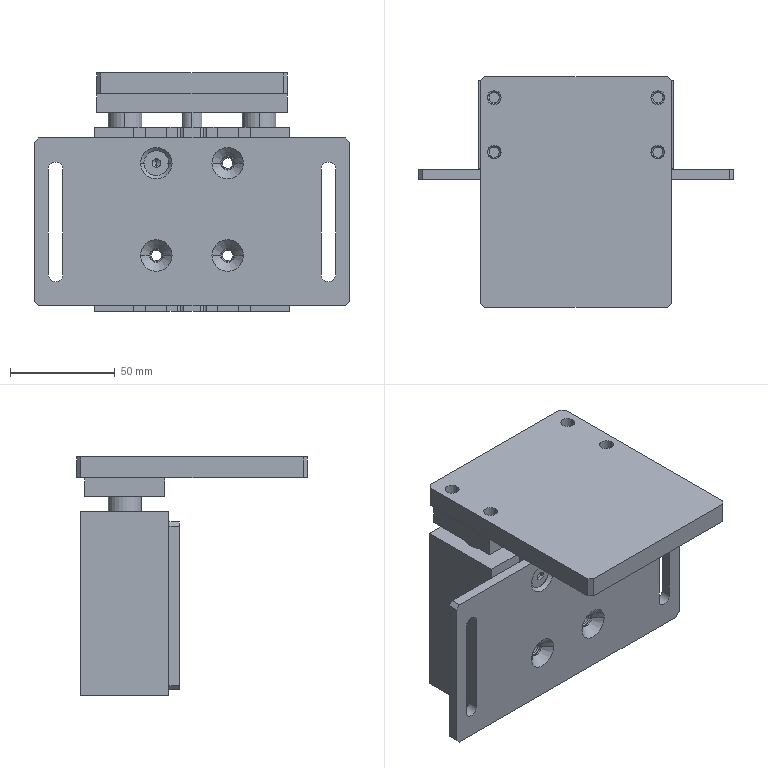Part | SolidWorks | 5 solids | 312 faces | box 150 x 110 x 113.5 mm | volume 470255 mm3 | plane 116 | cylinder 114 | cone 82 | commonest cylinder face diameters 4.917 x24 4 x18 6.6 x16 5.4 x8 8.566 x8 9.5 x8